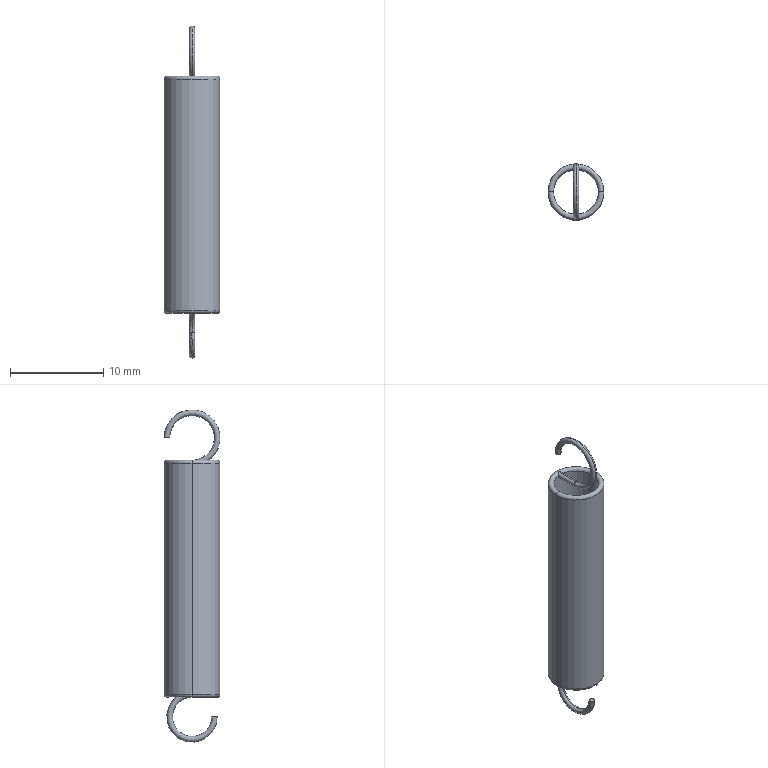Part | NX | features BREP 1 | 1 solid | 18 faces | box 6 x 6 x 35.6 mm | volume 265.602 mm3 | torus 8 | cylinder 8 | plane 2 | commonest cylinder face diameters 0.6 x4 4.8 x2 6 x2
STEP:
#1=CARTESIAN_POINT('',(-0.0001989,3.,2.7));
#2=VERTEX_POINT('',#1);
#3=CARTESIAN_POINT('',(0.0001989,2.4,2.7));
#4=VERTEX_POINT('',#3);
#5=CARTESIAN_POINT('',(0.,2.4,2.7));
#6=CARTESIAN_POINT('',(-0.1541,2.4,2.7));
#7=CARTESIAN_POINT('',(-0.4426,2.7,2.7));
#8=CARTESIAN_POINT('',(-0.1608,3.,2.7));
#9=CARTESIAN_POINT('',(-0.0001989,3.,2.7));
#10=B_SPLINE_CURVE_WITH_KNOTS('',3,(#5,#6,#7,#8,#9),.UNSPECIFIED.,.F.,.F.,(4,1,4),(0.,0.4999,0.9998),.UNSPECIFIED.);
#11=EDGE_CURVE('',#2,#4,#10,.F.);
#12=ORIENTED_EDGE('',*,*,#11,.F.);
#13=CARTESIAN_POINT('',(0.,3.,2.7));
#14=CARTESIAN_POINT('',(0.1527,3.,2.7));
#15=CARTESIAN_POINT('',(0.4428,2.701,2.7));
#16=CARTESIAN_POINT('',(0.1616,2.4,2.7));
#17=CARTESIAN_POINT('',(0.0001989,2.4,2.7));
#18=B_SPLINE_CURVE_WITH_KNOTS('',3,(#13,#14,#15,#16,#17),.UNSPECIFIED.,.F.,.F.,(4,1,4),(0.,0.4999,0.9998),.UNSPECIFIED.);
#19=EDGE_CURVE('',#4,#2,#18,.F.);
#20=ORIENTED_EDGE('',*,*,#19,.F.);
#21=EDGE_LOOP('',(#12,#20));
#22=FACE_BOUND('',#21,.T.);
#23=CARTESIAN_POINT('',(0.,2.7,2.7));
#24=DIRECTION('',(0.,0.,1.));
#25=DIRECTION('',(0.,-1.,0.));
#26=AXIS2_PLACEMENT_3D('',#23,#24,#25);
#27=PLANE('',#26);
#28=ADVANCED_FACE('',(#22),#27,.F.);
#29=CARTESIAN_POINT('',(-0.0001989,-2.7,-27.2));
#30=VERTEX_POINT('',#29);
#31=CARTESIAN_POINT('',(0.0001989,-2.1,-27.2));
#32=VERTEX_POINT('',#31);
#33=CARTESIAN_POINT('',(0.,-2.1,-27.2));
#34=CARTESIAN_POINT('',(-0.1541,-2.1,-27.2));
#35=CARTESIAN_POINT('',(-0.4426,-2.4,-27.2));
#36=CARTESIAN_POINT('',(-0.1608,-2.7,-27.2));
#37=CARTESIAN_POINT('',(-0.0001989,-2.7,-27.2));
#38=B_SPLINE_CURVE_WITH_KNOTS('',3,(#33,#34,#35,#36,#37),.UNSPECIFIED.,.F.,.F.,(4,1,4),(0.,0.4999,0.9998),.UNSPECIFIED.);
#39=EDGE_CURVE('',#30,#32,#38,.F.);
#40=ORIENTED_EDGE('',*,*,#39,.F.);
#41=CARTESIAN_POINT('',(0.,-2.7,-27.2));
#42=CARTESIAN_POINT('',(0.1527,-2.7,-27.2));
#43=CARTESIAN_POINT('',(0.4428,-2.401,-27.2));
#44=CARTESIAN_POINT('',(0.1616,-2.1,-27.2));
#45=CARTESIAN_POINT('',(0.0001989,-2.1,-27.2));
#46=B_SPLINE_CURVE_WITH_KNOTS('',3,(#41,#42,#43,#44,#45),.UNSPECIFIED.,.F.,.F.,(4,1,4),(0.,0.4999,0.9998),.UNSPECIFIED.);
#47=EDGE_CURVE('',#32,#30,#46,.F.);
#48=ORIENTED_EDGE('',*,*,#47,.F.);
#49=EDGE_LOOP('',(#40,#48));
#50=FACE_BOUND('',#49,.T.);
#51=CARTESIAN_POINT('',(0.,-2.4,-27.2));
#52=DIRECTION('',(0.,0.,1.));
#53=DIRECTION('',(0.,-1.,0.));
#54=AXIS2_PLACEMENT_3D('',#51,#52,#53);
#55=PLANE('',#54);
#56=ADVANCED_FACE('',(#50),#55,.T.);
#57=CARTESIAN_POINT('',(0.,0.,0.3));
#58=VERTEX_POINT('',#57);
#59=CARTESIAN_POINT('',(0.,0.,2.7));
#60=DIRECTION('',(1.,0.,0.));
#61=DIRECTION('',(0.,0.,-1.));
#62=AXIS2_PLACEMENT_3D('',#59,#60,#61);
#63=CIRCLE('',#62,2.4);
#64=EDGE_CURVE('',#4,#58,#63,.T.);
#65=ORIENTED_EDGE('',*,*,#64,.F.);
#66=ORIENTED_EDGE('',*,*,#19,.T.);
#67=CARTESIAN_POINT('',(0.,0.,-0.3));
#68=VERTEX_POINT('',#67);
#69=CARTESIAN_POINT('',(0.,0.,2.7));
#70=DIRECTION('',(1.,0.,0.));
#71=DIRECTION('',(0.,0.,-1.));
#72=AXIS2_PLACEMENT_3D('',#69,#70,#71);
#73=CIRCLE('',#72,3.);
#74=EDGE_CURVE('',#2,#68,#73,.T.);
#75=ORIENTED_EDGE('',*,*,#74,.T.);
#76=CARTESIAN_POINT('',(0.,0.,0.));
#77=DIRECTION('',(0.,1.,0.));
#78=DIRECTION('',(0.,0.,1.));
#79=AXIS2_PLACEMENT_3D('',#76,#77,#78);
#80=CIRCLE('',#79,0.3);
#81=EDGE_CURVE('',#58,#68,#80,.T.);
#82=ORIENTED_EDGE('',*,*,#81,.F.);
#83=EDGE_LOOP('',(#65,#66,#75,#82));
#84=FACE_BOUND('',#83,.T.);
#85=CARTESIAN_POINT('',(0.,0.,2.7));
#86=DIRECTION('',(1.,0.,0.));
#87=DIRECTION('',(0.,0.,-1.));
#88=AXIS2_PLACEMENT_3D('',#85,#86,#87);
#89=TOROIDAL_SURFACE('',#88,2.7,0.3);
#90=ADVANCED_FACE('',(#84),#89,.T.);
#91=CARTESIAN_POINT('',(0.,0.,-25.1));
#92=VERTEX_POINT('',#91);
#93=CARTESIAN_POINT('',(0.,0.,-27.2));
#94=DIRECTION('',(-1.,0.,0.));
#95=DIRECTION('',(0.,0.,1.));
#96=AXIS2_PLACEMENT_3D('',#93,#94,#95);
#97=CIRCLE('',#96,2.1);
#98=EDGE_CURVE('',#92,#32,#97,.T.);
#99=ORIENTED_EDGE('',*,*,#98,.F.);
#100=CARTESIAN_POINT('',(0.,0.,-24.5));
#101=VERTEX_POINT('',#100);
#102=CARTESIAN_POINT('',(0.,0.,-24.8));
#103=DIRECTION('',(0.,-1.,0.));
#104=DIRECTION('',(0.,0.,-1.));
#105=AXIS2_PLACEMENT_3D('',#102,#103,#104);
#106=CIRCLE('',#105,0.3);
#107=EDGE_CURVE('',#101,#92,#106,.T.);
#108=ORIENTED_EDGE('',*,*,#107,.F.);
#109=CARTESIAN_POINT('',(0.,0.,-27.2));
#110=DIRECTION('',(-1.,0.,0.));
#111=DIRECTION('',(0.,0.,1.));
#112=AXIS2_PLACEMENT_3D('',#109,#110,#111);
#113=CIRCLE('',#112,2.7);
#114=EDGE_CURVE('',#101,#30,#113,.T.);
#115=ORIENTED_EDGE('',*,*,#114,.T.);
#116=ORIENTED_EDGE('',*,*,#39,.T.);
#117=EDGE_LOOP('',(#99,#108,#115,#116));
#118=FACE_BOUND('',#117,.T.);
#119=CARTESIAN_POINT('',(0.,0.,-27.2));
#120=DIRECTION('',(1.,0.,0.));
#121=DIRECTION('',(0.,1.,0.));
#122=AXIS2_PLACEMENT_3D('',#119,#120,#121);
#123=TOROIDAL_SURFACE('',#122,2.4,0.3);
#124=ADVANCED_FACE('',(#118),#123,.T.);
#125=CARTESIAN_POINT('',(0.,2.4,-0.3));
#126=VERTEX_POINT('',#125);
#127=CARTESIAN_POINT('',(0.,2.7,-0.3));
#128=DIRECTION('',(0.,1.,0.));
#129=VECTOR('',#128,1000.);
#130=LINE('',#127,#129);
#131=EDGE_CURVE('',#126,#68,#130,.F.);
#132=ORIENTED_EDGE('',*,*,#131,.T.);
#133=CARTESIAN_POINT('',(0.,0.,0.));
#134=DIRECTION('',(0.,1.,0.));
#135=DIRECTION('',(0.,0.,1.));
#136=AXIS2_PLACEMENT_3D('',#133,#134,#135);
#137=CIRCLE('',#136,0.3);
#138=EDGE_CURVE('',#68,#58,#137,.T.);
#139=ORIENTED_EDGE('',*,*,#138,.T.);
#140=CARTESIAN_POINT('',(0.,2.7,0.3));
#141=VERTEX_POINT('',#140);
#142=CARTESIAN_POINT('',(0.,2.7,0.3));
#143=DIRECTION('',(0.,1.,0.));
#144=VECTOR('',#143,1000.);
#145=LINE('',#142,#144);
#146=EDGE_CURVE('',#141,#58,#145,.F.);
#147=ORIENTED_EDGE('',*,*,#146,.F.);
#148=CARTESIAN_POINT('',(-0.3,2.381,0.0001807));
#149=VERTEX_POINT('',#148);
#150=CARTESIAN_POINT('',(0.,2.7,0.3));
#151=CARTESIAN_POINT('',(-0.0455,2.655,0.3));
#152=CARTESIAN_POINT('',(-0.2137,2.48,0.2633));
#153=CARTESIAN_POINT('',(-0.2999,2.381,0.09145));
#154=CARTESIAN_POINT('',(-0.3,2.381,0.0001807));
#155=B_SPLINE_CURVE_WITH_KNOTS('',3,(#150,#151,#152,#153,#154),.UNSPECIFIED.,.F.,.F.,(4,1,4),(0.,0.4998,0.9997),.UNSPECIFIED.);
#156=EDGE_CURVE('',#149,#141,#155,.F.);
#157=ORIENTED_EDGE('',*,*,#156,.F.);
#158=CARTESIAN_POINT('',(-0.3,2.381,0.));
#159=CARTESIAN_POINT('',(-0.3,2.381,-0.05688));
#160=CARTESIAN_POINT('',(-0.2455,2.391,-0.246));
#161=CARTESIAN_POINT('',(-0.05727,2.4,-0.3));
#162=CARTESIAN_POINT('',(0.,2.4,-0.3));
#163=B_SPLINE_CURVE_WITH_KNOTS('',3,(#158,#159,#160,#161,#162),.UNSPECIFIED.,.F.,.F.,(4,1,4),(0.,0.5,1.),.UNSPECIFIED.);
#164=EDGE_CURVE('',#149,#126,#163,.T.);
#165=ORIENTED_EDGE('',*,*,#164,.T.);
#166=EDGE_LOOP('',(#132,#139,#147,#157,#165));
#167=FACE_BOUND('',#166,.T.);
#168=CARTESIAN_POINT('',(0.,2.7,0.));
#169=DIRECTION('',(0.,1.,0.));
#170=DIRECTION('',(0.,0.,1.));
#171=AXIS2_PLACEMENT_3D('',#168,#169,#170);
#172=CYLINDRICAL_SURFACE('',#171,0.3);
#173=ADVANCED_FACE('',(#167),#172,.T.);
#174=CARTESIAN_POINT('',(-2.4,0.,0.));
#175=VERTEX_POINT('',#174);
#176=CARTESIAN_POINT('',(-2.4,0.,-24.8));
#177=VERTEX_POINT('',#176);
#178=CARTESIAN_POINT('',(-2.4,0.,-25.1));
#179=DIRECTION('',(0.,0.,1.));
#180=VECTOR('',#179,1000.);
#181=LINE('',#178,#180);
#182=EDGE_CURVE('',#175,#177,#181,.F.);
#183=ORIENTED_EDGE('',*,*,#182,.T.);
#184=CARTESIAN_POINT('',(2.4,0.,-24.8));
#185=VERTEX_POINT('',#184);
#186=CARTESIAN_POINT('',(0.,0.,-24.8));
#187=DIRECTION('',(0.,0.,1.));
#188=DIRECTION('',(-1.,0.,0.));
#189=AXIS2_PLACEMENT_3D('',#186,#187,#188);
#190=CIRCLE('',#189,2.4);
#191=EDGE_CURVE('',#185,#177,#190,.T.);
#192=ORIENTED_EDGE('',*,*,#191,.F.);
#193=CARTESIAN_POINT('',(2.4,0.,0.));
#194=VERTEX_POINT('',#193);
#195=CARTESIAN_POINT('',(2.4,0.,-25.1));
#196=DIRECTION('',(0.,0.,1.));
#197=VECTOR('',#196,1000.);
#198=LINE('',#195,#197);
#199=EDGE_CURVE('',#194,#185,#198,.F.);
#200=ORIENTED_EDGE('',*,*,#199,.F.);
#201=CARTESIAN_POINT('',(0.3,2.381,0.0001773));
#202=VERTEX_POINT('',#201);
#203=CARTESIAN_POINT('',(0.,0.,0.));
#204=DIRECTION('',(0.,0.,-1.));
#205=DIRECTION('',(-1.,0.,0.));
#206=AXIS2_PLACEMENT_3D('',#203,#204,#205);
#207=CIRCLE('',#206,2.4);
#208=EDGE_CURVE('',#202,#194,#207,.T.);
#209=ORIENTED_EDGE('',*,*,#208,.F.);
#210=CARTESIAN_POINT('',(0.3,2.381,0.));
#211=CARTESIAN_POINT('',(0.2993,2.381,-0.1601));
#212=CARTESIAN_POINT('',(0.157,2.4,-0.3));
#213=CARTESIAN_POINT('',(0.,2.4,-0.3));
#214=B_SPLINE_CURVE_WITH_KNOTS('',3,(#210,#211,#212,#213),.UNSPECIFIED.,.F.,.F.,(4,4),(0.,1.),.UNSPECIFIED.);
#215=EDGE_CURVE('',#126,#202,#214,.F.);
#216=ORIENTED_EDGE('',*,*,#215,.F.);
#217=ORIENTED_EDGE('',*,*,#164,.F.);
#218=CARTESIAN_POINT('',(0.,0.,0.));
#219=DIRECTION('',(0.,0.,-1.));
#220=DIRECTION('',(-1.,0.,0.));
#221=AXIS2_PLACEMENT_3D('',#218,#219,#220);
#222=CIRCLE('',#221,2.4);
#223=EDGE_CURVE('',#175,#149,#222,.T.);
#224=ORIENTED_EDGE('',*,*,#223,.F.);
#225=EDGE_LOOP('',(#183,#192,#200,#209,#216,#217,#224));
#226=FACE_BOUND('',#225,.T.);
#227=CARTESIAN_POINT('',(0.,0.,-25.1));
#228=DIRECTION('',(0.,0.,1.));
#229=DIRECTION('',(1.,0.,0.));
#230=AXIS2_PLACEMENT_3D('',#227,#228,#229);
#231=CYLINDRICAL_SURFACE('',#230,2.4);
#232=ADVANCED_FACE('',(#226),#231,.F.);
#233=CARTESIAN_POINT('',(0.,-2.4,-24.5));
#234=VERTEX_POINT('',#233);
#235=CARTESIAN_POINT('',(0.,-2.7,-24.5));
#236=DIRECTION('',(0.,-1.,0.));
#237=VECTOR('',#236,1000.);
#238=LINE('',#235,#237);
#239=EDGE_CURVE('',#101,#234,#238,.T.);
#240=ORIENTED_EDGE('',*,*,#239,.F.);
#241=ORIENTED_EDGE('',*,*,#107,.T.);
#242=CARTESIAN_POINT('',(0.,-2.7,-25.1));
#243=VERTEX_POINT('',#242);
#244=CARTESIAN_POINT('',(0.,-2.7,-25.1));
#245=DIRECTION('',(0.,-1.,0.));
#246=VECTOR('',#245,1000.);
#247=LINE('',#244,#246);
#248=EDGE_CURVE('',#92,#243,#247,.T.);
#249=ORIENTED_EDGE('',*,*,#248,.T.);
#250=CARTESIAN_POINT('',(-0.3,-2.381,-24.8));
#251=VERTEX_POINT('',#250);
#252=CARTESIAN_POINT('',(0.,-2.7,-25.1));
#253=CARTESIAN_POINT('',(-0.0455,-2.655,-25.1));
#254=CARTESIAN_POINT('',(-0.2137,-2.48,-25.063));
#255=CARTESIAN_POINT('',(-0.2999,-2.381,-24.891));
#256=CARTESIAN_POINT('',(-0.3,-2.381,-24.8));
#257=B_SPLINE_CURVE_WITH_KNOTS('',3,(#252,#253,#254,#255,#256),.UNSPECIFIED.,.F.,.F.,(4,1,4),(0.,0.4998,0.9997),.UNSPECIFIED.);
#258=EDGE_CURVE('',#251,#243,#257,.F.);
#259=ORIENTED_EDGE('',*,*,#258,.F.);
#260=CARTESIAN_POINT('',(-0.3,-2.381,-24.8));
#261=CARTESIAN_POINT('',(-0.3,-2.381,-24.743));
#262=CARTESIAN_POINT('',(-0.2455,-2.391,-24.554));
#263=CARTESIAN_POINT('',(-0.05727,-2.4,-24.5));
#264=CARTESIAN_POINT('',(0.,-2.4,-24.5));
#265=B_SPLINE_CURVE_WITH_KNOTS('',3,(#260,#261,#262,#263,#264),.UNSPECIFIED.,.F.,.F.,(4,1,4),(0.,0.5,1.),.UNSPECIFIED.);
#266=EDGE_CURVE('',#251,#234,#265,.T.);
#267=ORIENTED_EDGE('',*,*,#266,.T.);
#268=EDGE_LOOP('',(#240,#241,#249,#259,#267));
#269=FACE_BOUND('',#268,.T.);
#270=CARTESIAN_POINT('',(0.,-2.7,-24.8));
#271=DIRECTION('',(0.,-1.,0.));
#272=DIRECTION('',(0.,0.,-1.));
#273=AXIS2_PLACEMENT_3D('',#270,#271,#272);
#274=CYLINDRICAL_SURFACE('',#273,0.3);
#275=ADVANCED_FACE('',(#269),#274,.T.);
#276=CARTESIAN_POINT('',(3.,0.,0.));
#277=VERTEX_POINT('',#276);
#278=CARTESIAN_POINT('',(2.7,0.,0.));
#279=DIRECTION('',(0.,-1.,0.));
#280=DIRECTION('',(1.,0.,0.));
#281=AXIS2_PLACEMENT_3D('',#278,#279,#280);
#282=CIRCLE('',#281,0.3);
#283=EDGE_CURVE('',#277,#194,#282,.T.);
#284=ORIENTED_EDGE('',*,*,#283,.F.);
#285=CARTESIAN_POINT('',(-3.,0.,0.));
#286=VERTEX_POINT('',#285);
#287=CARTESIAN_POINT('',(0.,0.,0.));
#288=DIRECTION('',(0.,0.,-1.));
#289=DIRECTION('',(1.,0.,0.));
#290=AXIS2_PLACEMENT_3D('',#287,#288,#289);
#291=CIRCLE('',#290,3.);
#292=EDGE_CURVE('',#286,#277,#291,.T.);
#293=ORIENTED_EDGE('',*,*,#292,.F.);
#294=CARTESIAN_POINT('',(-2.7,0.,0.));
#295=DIRECTION('',(0.,1.,0.));
#296=DIRECTION('',(-1.,0.,0.));
#297=AXIS2_PLACEMENT_3D('',#294,#295,#296);
#298=CIRCLE('',#297,0.3);
#299=EDGE_CURVE('',#286,#175,#298,.T.);
#300=ORIENTED_EDGE('',*,*,#299,.T.);
#301=ORIENTED_EDGE('',*,*,#223,.T.);
#302=ORIENTED_EDGE('',*,*,#156,.T.);
#303=CARTESIAN_POINT('',(0.3,2.381,0.0001773));
#304=CARTESIAN_POINT('',(0.2999,2.381,0.0911));
#305=CARTESIAN_POINT('',(0.2207,2.47,0.2218));
#306=CARTESIAN_POINT('',(0.1128,2.586,0.2876));
#307=CARTESIAN_POINT('',(0.01141,2.689,0.3));
#308=CARTESIAN_POINT('',(0.,2.7,0.3));
#309=B_SPLINE_CURVE_WITH_KNOTS('',3,(#303,#304,#305,#306,#307,#308),.UNSPECIFIED.,.F.,.F.,(4,1,1,4),(0.000325,0.5002,0.7501,1.),.UNSPECIFIED.);
#310=EDGE_CURVE('',#141,#202,#309,.F.);
#311=ORIENTED_EDGE('',*,*,#310,.T.);
#312=ORIENTED_EDGE('',*,*,#208,.T.);
#313=EDGE_LOOP('',(#284,#293,#300,#301,#302,#311,#312));
#314=FACE_BOUND('',#313,.T.);
#315=CARTESIAN_POINT('',(0.,0.,0.));
#316=DIRECTION('',(0.,0.,1.));
#317=DIRECTION('',(0.,-1.,0.));
#318=AXIS2_PLACEMENT_3D('',#315,#316,#317);
#319=TOROIDAL_SURFACE('',#318,2.7,0.3);
#320=ADVANCED_FACE('',(#314),#319,.T.);
#321=CARTESIAN_POINT('',(3.,0.,-24.8));
#322=VERTEX_POINT('',#321);
#323=CARTESIAN_POINT('',(2.7,0.,-24.8));
#324=DIRECTION('',(0.,-1.,0.));
#325=DIRECTION('',(1.,0.,0.));
#326=AXIS2_PLACEMENT_3D('',#323,#324,#325);
#327=CIRCLE('',#326,0.3);
#328=EDGE_CURVE('',#185,#322,#327,.T.);
#329=ORIENTED_EDGE('',*,*,#328,.F.);
#330=ORIENTED_EDGE('',*,*,#191,.T.);
#331=CARTESIAN_POINT('',(-3.,0.,-24.8));
#332=VERTEX_POINT('',#331);
#333=CARTESIAN_POINT('',(-2.7,0.,-24.8));
#334=DIRECTION('',(0.,1.,0.));
#335=DIRECTION('',(-1.,0.,0.));
#336=AXIS2_PLACEMENT_3D('',#333,#334,#335);
#337=CIRCLE('',#336,0.3);
#338=EDGE_CURVE('',#177,#332,#337,.T.);
#339=ORIENTED_EDGE('',*,*,#338,.T.);
#340=CARTESIAN_POINT('',(0.,0.,-24.8));
#341=DIRECTION('',(0.,0.,1.));
#342=DIRECTION('',(1.,0.,0.));
#343=AXIS2_PLACEMENT_3D('',#340,#341,#342);
#344=CIRCLE('',#343,3.);
#345=EDGE_CURVE('',#322,#332,#344,.T.);
#346=ORIENTED_EDGE('',*,*,#345,.F.);
#347=EDGE_LOOP('',(#329,#330,#339,#346));
#348=FACE_BOUND('',#347,.T.);
#349=CARTESIAN_POINT('',(0.,0.,-24.8));
#350=DIRECTION('',(0.,0.,1.));
#351=DIRECTION('',(1.,0.,0.));
#352=AXIS2_PLACEMENT_3D('',#349,#350,#351);
#353=TOROIDAL_SURFACE('',#352,2.7,0.3);
#354=ADVANCED_FACE('',(#348),#353,.T.);
#355=CARTESIAN_POINT('',(-3.,0.,-25.1));
#356=DIRECTION('',(0.,0.,1.));
#357=VECTOR('',#356,1000.);
#358=LINE('',#355,#357);
#359=EDGE_CURVE('',#286,#332,#358,.F.);
#360=ORIENTED_EDGE('',*,*,#359,.T.);
#361=CARTESIAN_POINT('',(0.,0.,-24.8));
#362=DIRECTION('',(0.,0.,1.));
#363=DIRECTION('',(1.,0.,0.));
#364=AXIS2_PLACEMENT_3D('',#361,#362,#363);
#365=CIRCLE('',#364,3.);
#366=EDGE_CURVE('',#332,#322,#365,.T.);
#367=ORIENTED_EDGE('',*,*,#366,.T.);
#368=CARTESIAN_POINT('',(3.,0.,-25.1));
#369=DIRECTION('',(0.,0.,1.));
#370=VECTOR('',#369,1000.);
#371=LINE('',#368,#370);
#372=EDGE_CURVE('',#277,#322,#371,.F.);
#373=ORIENTED_EDGE('',*,*,#372,.F.);
#374=CARTESIAN_POINT('',(0.,0.,0.));
#375=DIRECTION('',(0.,0.,-1.));
#376=DIRECTION('',(1.,0.,0.));
#377=AXIS2_PLACEMENT_3D('',#374,#375,#376);
#378=CIRCLE('',#377,3.);
#379=EDGE_CURVE('',#277,#286,#378,.T.);
#380=ORIENTED_EDGE('',*,*,#379,.T.);
#381=EDGE_LOOP('',(#360,#367,#373,#380));
#382=FACE_BOUND('',#381,.T.);
#383=CARTESIAN_POINT('',(0.,0.,-25.1));
#384=DIRECTION('',(0.,0.,1.));
#385=DIRECTION('',(1.,0.,0.));
#386=AXIS2_PLACEMENT_3D('',#383,#384,#385);
#387=CYLINDRICAL_SURFACE('',#386,3.);
#388=ADVANCED_FACE('',(#382),#387,.T.);
#389=ORIENTED_EDGE('',*,*,#11,.T.);
#390=ORIENTED_EDGE('',*,*,#64,.T.);
#391=ORIENTED_EDGE('',*,*,#138,.F.);
#392=ORIENTED_EDGE('',*,*,#74,.F.);
#393=EDGE_LOOP('',(#389,#390,#391,#392));
#394=FACE_BOUND('',#393,.T.);
#395=CARTESIAN_POINT('',(0.,0.,2.7));
#396=DIRECTION('',(1.,0.,0.));
#397=DIRECTION('',(0.,0.,-1.));
#398=AXIS2_PLACEMENT_3D('',#395,#396,#397);
#399=TOROIDAL_SURFACE('',#398,2.7,0.3);
#400=ADVANCED_FACE('',(#394),#399,.T.);
#401=CARTESIAN_POINT('',(0.,0.,-24.8));
#402=DIRECTION('',(0.,-1.,0.));
#403=DIRECTION('',(0.,0.,-1.));
#404=AXIS2_PLACEMENT_3D('',#401,#402,#403);
#405=CIRCLE('',#404,0.3);
#406=EDGE_CURVE('',#92,#101,#405,.T.);
#407=ORIENTED_EDGE('',*,*,#406,.F.);
#408=ORIENTED_EDGE('',*,*,#98,.T.);
#409=ORIENTED_EDGE('',*,*,#47,.T.);
#410=ORIENTED_EDGE('',*,*,#114,.F.);
#411=EDGE_LOOP('',(#407,#408,#409,#410));
#412=FACE_BOUND('',#411,.T.);
#413=CARTESIAN_POINT('',(0.,0.,-27.2));
#414=DIRECTION('',(1.,0.,0.));
#415=DIRECTION('',(0.,0.,-1.));
#416=AXIS2_PLACEMENT_3D('',#413,#414,#415);
#417=TOROIDAL_SURFACE('',#416,2.4,0.3);
#418=ADVANCED_FACE('',(#412),#417,.T.);
#419=ORIENTED_EDGE('',*,*,#81,.T.);
#420=ORIENTED_EDGE('',*,*,#131,.F.);
#421=ORIENTED_EDGE('',*,*,#215,.T.);
#422=ORIENTED_EDGE('',*,*,#310,.F.);
#423=ORIENTED_EDGE('',*,*,#146,.T.);
#424=EDGE_LOOP('',(#419,#420,#421,#422,#423));
#425=FACE_BOUND('',#424,.T.);
#426=CARTESIAN_POINT('',(0.,2.7,0.));
#427=DIRECTION('',(0.,1.,0.));
#428=DIRECTION('',(0.,0.,1.));
#429=AXIS2_PLACEMENT_3D('',#426,#427,#428);
#430=CYLINDRICAL_SURFACE('',#429,0.3);
#431=ADVANCED_FACE('',(#425),#430,.T.);
#432=CARTESIAN_POINT('',(0.,0.,-24.8));
#433=DIRECTION('',(0.,0.,1.));
#434=DIRECTION('',(-1.,0.,0.));
#435=AXIS2_PLACEMENT_3D('',#432,#433,#434);
#436=CIRCLE('',#435,2.4);
#437=EDGE_CURVE('',#177,#251,#436,.T.);
#438=ORIENTED_EDGE('',*,*,#437,.F.);
#439=ORIENTED_EDGE('',*,*,#182,.F.);
#440=CARTESIAN_POINT('',(0.,0.,0.));
#441=DIRECTION('',(0.,0.,-1.));
#442=DIRECTION('',(-1.,0.,0.));
#443=AXIS2_PLACEMENT_3D('',#440,#441,#442);
#444=CIRCLE('',#443,2.4);
#445=EDGE_CURVE('',#194,#175,#444,.T.);
#446=ORIENTED_EDGE('',*,*,#445,.F.);
#447=ORIENTED_EDGE('',*,*,#199,.T.);
#448=CARTESIAN_POINT('',(0.3,-2.381,-24.8));
#449=VERTEX_POINT('',#448);
#450=CARTESIAN_POINT('',(0.,0.,-24.8));
#451=DIRECTION('',(0.,0.,1.));
#452=DIRECTION('',(-1.,0.,0.));
#453=AXIS2_PLACEMENT_3D('',#450,#451,#452);
#454=CIRCLE('',#453,2.4);
#455=EDGE_CURVE('',#449,#185,#454,.T.);
#456=ORIENTED_EDGE('',*,*,#455,.F.);
#457=CARTESIAN_POINT('',(0.3,-2.381,-24.8));
#458=CARTESIAN_POINT('',(0.2993,-2.381,-24.64));
#459=CARTESIAN_POINT('',(0.157,-2.4,-24.5));
#460=CARTESIAN_POINT('',(0.,-2.4,-24.5));
#461=B_SPLINE_CURVE_WITH_KNOTS('',3,(#457,#458,#459,#460),.UNSPECIFIED.,.F.,.F.,(4,4),(0.,1.),.UNSPECIFIED.);
#462=EDGE_CURVE('',#234,#449,#461,.F.);
#463=ORIENTED_EDGE('',*,*,#462,.F.);
#464=ORIENTED_EDGE('',*,*,#266,.F.);
#465=EDGE_LOOP('',(#438,#439,#446,#447,#456,#463,#464));
#466=FACE_BOUND('',#465,.T.);
#467=CARTESIAN_POINT('',(0.,0.,-25.1));
#468=DIRECTION('',(0.,0.,1.));
#469=DIRECTION('',(1.,0.,0.));
#470=AXIS2_PLACEMENT_3D('',#467,#468,#469);
#471=CYLINDRICAL_SURFACE('',#470,2.4);
#472=ADVANCED_FACE('',(#466),#471,.F.);
#473=ORIENTED_EDGE('',*,*,#406,.T.);
#474=ORIENTED_EDGE('',*,*,#239,.T.);
#475=ORIENTED_EDGE('',*,*,#462,.T.);
#476=CARTESIAN_POINT('',(0.3,-2.381,-24.8));
#477=CARTESIAN_POINT('',(0.2999,-2.381,-24.891));
#478=CARTESIAN_POINT('',(0.2207,-2.47,-25.022));
#479=CARTESIAN_POINT('',(0.1128,-2.586,-25.088));
#480=CARTESIAN_POINT('',(0.01141,-2.689,-25.1));
#481=CARTESIAN_POINT('',(0.,-2.7,-25.1));
#482=B_SPLINE_CURVE_WITH_KNOTS('',3,(#476,#477,#478,#479,#480,#481),.UNSPECIFIED.,.F.,.F.,(4,1,1,4),(0.000325,0.5002,0.7501,1.),.UNSPECIFIED.);
#483=EDGE_CURVE('',#243,#449,#482,.F.);
#484=ORIENTED_EDGE('',*,*,#483,.F.);
#485=ORIENTED_EDGE('',*,*,#248,.F.);
#486=EDGE_LOOP('',(#473,#474,#475,#484,#485));
#487=FACE_BOUND('',#486,.T.);
#488=CARTESIAN_POINT('',(0.,-2.7,-24.8));
#489=DIRECTION('',(0.,-1.,0.));
#490=DIRECTION('',(0.,0.,-1.));
#491=AXIS2_PLACEMENT_3D('',#488,#489,#490);
#492=CYLINDRICAL_SURFACE('',#491,0.3);
#493=ADVANCED_FACE('',(#487),#492,.T.);
#494=ORIENTED_EDGE('',*,*,#345,.T.);
#495=ORIENTED_EDGE('',*,*,#359,.F.);
#496=ORIENTED_EDGE('',*,*,#292,.T.);
#497=ORIENTED_EDGE('',*,*,#372,.T.);
#498=EDGE_LOOP('',(#494,#495,#496,#497));
#499=FACE_BOUND('',#498,.T.);
#500=CARTESIAN_POINT('',(0.,0.,-25.1));
#501=DIRECTION('',(0.,0.,1.));
#502=DIRECTION('',(1.,0.,0.));
#503=AXIS2_PLACEMENT_3D('',#500,#501,#502);
#504=CYLINDRICAL_SURFACE('',#503,3.);
#505=ADVANCED_FACE('',(#499),#504,.T.);
#506=ORIENTED_EDGE('',*,*,#379,.F.);
#507=ORIENTED_EDGE('',*,*,#283,.T.);
#508=ORIENTED_EDGE('',*,*,#445,.T.);
#509=ORIENTED_EDGE('',*,*,#299,.F.);
#510=EDGE_LOOP('',(#506,#507,#508,#509));
#511=FACE_BOUND('',#510,.T.);
#512=CARTESIAN_POINT('',(0.,0.,0.));
#513=DIRECTION('',(0.,0.,1.));
#514=DIRECTION('',(1.,0.,0.));
#515=AXIS2_PLACEMENT_3D('',#512,#513,#514);
#516=TOROIDAL_SURFACE('',#515,2.7,0.3);
#517=ADVANCED_FACE('',(#511),#516,.T.);
#518=ORIENTED_EDGE('',*,*,#455,.T.);
#519=ORIENTED_EDGE('',*,*,#328,.T.);
#520=ORIENTED_EDGE('',*,*,#366,.F.);
#521=ORIENTED_EDGE('',*,*,#338,.F.);
#522=ORIENTED_EDGE('',*,*,#437,.T.);
#523=ORIENTED_EDGE('',*,*,#258,.T.);
#524=ORIENTED_EDGE('',*,*,#483,.T.);
#525=EDGE_LOOP('',(#518,#519,#520,#521,#522,#523,#524));
#526=FACE_BOUND('',#525,.T.);
#527=CARTESIAN_POINT('',(0.,0.,-24.8));
#528=DIRECTION('',(0.,0.,1.));
#529=DIRECTION('',(1.,0.,0.));
#530=AXIS2_PLACEMENT_3D('',#527,#528,#529);
#531=TOROIDAL_SURFACE('',#530,2.7,0.3);
#532=ADVANCED_FACE('',(#526),#531,.T.);
#533=CLOSED_SHELL('',(#28,#56,#90,#124,#173,#232,#275,#320,#354,#388,#400,#418,#431,#472,#493,#505,#517,#532));
#534=MANIFOLD_SOLID_BREP('',#533);
#535=(LENGTH_UNIT()NAMED_UNIT(*)SI_UNIT(.MILLI.,.METRE.));
#536=UNCERTAINTY_MEASURE_WITH_UNIT(LENGTH_MEASURE(0.0508),#535,'','');
#537=(NAMED_UNIT(*)PLANE_ANGLE_UNIT()SI_UNIT($,.RADIAN.));
#538=(NAMED_UNIT(*)SI_UNIT($,.STERADIAN.)SOLID_ANGLE_UNIT());
#539=(GEOMETRIC_REPRESENTATION_CONTEXT(3)GLOBAL_UNCERTAINTY_ASSIGNED_CONTEXT((#536))GLOBAL_UNIT_ASSIGNED_CONTEXT((#535,#537,#538))REPRESENTATION_CONTEXT('',''));
#540=ADVANCED_BREP_SHAPE_REPRESENTATION('',(#534),#539);